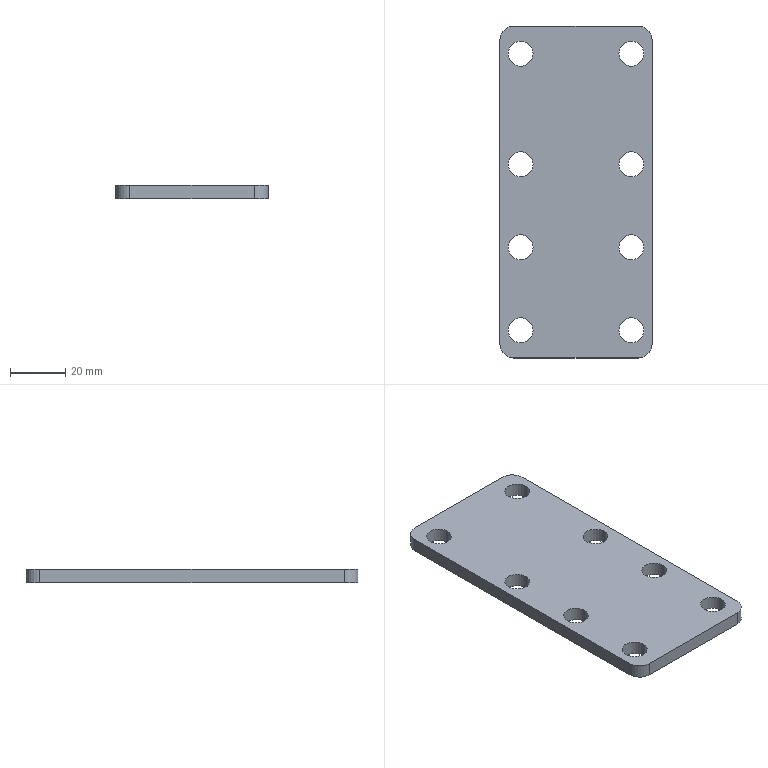Part | SolidWorks | features BaseBody 1 | 1 solid | 26 faces | box 55 x 120 x 5 mm | volume 30348 mm3 | cylinder 20 | plane 6 | commonest cylinder face diameters 9 x16 10 x4
STEP:
#1=CARTESIAN_POINT('',(3.,-10.,0.));
#2=VERTEX_POINT('',#1);
#3=CARTESIAN_POINT('',(12.,-10.,0.));
#4=VERTEX_POINT('',#3);
#5=CARTESIAN_POINT('',(7.5,-10.,0.));
#6=DIRECTION('',(0.,0.,1.));
#7=DIRECTION('',(1.,0.,0.));
#8=AXIS2_PLACEMENT_3D('',#5,#6,#7);
#9=CIRCLE('',#8,4.5);
#10=EDGE_CURVE('',#2,#4,#9,.T.);
#11=ORIENTED_EDGE('',*,*,#10,.F.);
#12=CARTESIAN_POINT('',(3.,-10.,5.));
#13=VERTEX_POINT('',#12);
#14=CARTESIAN_POINT('',(3.,-10.,5.));
#15=DIRECTION('',(0.,0.,1.));
#16=VECTOR('',#15,1000.);
#17=LINE('',#14,#16);
#18=EDGE_CURVE('',#2,#13,#17,.T.);
#19=ORIENTED_EDGE('',*,*,#18,.T.);
#20=CARTESIAN_POINT('',(12.,-10.,5.));
#21=VERTEX_POINT('',#20);
#22=CARTESIAN_POINT('',(7.5,-10.,5.));
#23=DIRECTION('',(0.,0.,1.));
#24=DIRECTION('',(1.,0.,0.));
#25=AXIS2_PLACEMENT_3D('',#22,#23,#24);
#26=CIRCLE('',#25,4.5);
#27=EDGE_CURVE('',#13,#21,#26,.T.);
#28=ORIENTED_EDGE('',*,*,#27,.T.);
#29=CARTESIAN_POINT('',(12.,-10.,5.));
#30=DIRECTION('',(0.,0.,1.));
#31=VECTOR('',#30,1000.);
#32=LINE('',#29,#31);
#33=EDGE_CURVE('',#4,#21,#32,.T.);
#34=ORIENTED_EDGE('',*,*,#33,.F.);
#35=EDGE_LOOP('',(#11,#19,#28,#34));
#36=FACE_OUTER_BOUND('',#35,.T.);
#37=CARTESIAN_POINT('',(7.5,-10.,5.));
#38=DIRECTION('',(0.,0.,1.));
#39=DIRECTION('',(1.,0.,0.));
#40=AXIS2_PLACEMENT_3D('',#37,#38,#39);
#41=CYLINDRICAL_SURFACE('',#40,4.5);
#42=ADVANCED_FACE('',(#36),#41,.F.);
#43=CARTESIAN_POINT('',(43.,-10.,0.));
#44=VERTEX_POINT('',#43);
#45=CARTESIAN_POINT('',(52.,-10.,0.));
#46=VERTEX_POINT('',#45);
#47=CARTESIAN_POINT('',(47.5,-10.,0.));
#48=DIRECTION('',(0.,0.,1.));
#49=DIRECTION('',(1.,0.,0.));
#50=AXIS2_PLACEMENT_3D('',#47,#48,#49);
#51=CIRCLE('',#50,4.5);
#52=EDGE_CURVE('',#44,#46,#51,.T.);
#53=ORIENTED_EDGE('',*,*,#52,.F.);
#54=CARTESIAN_POINT('',(43.,-10.,5.));
#55=VERTEX_POINT('',#54);
#56=CARTESIAN_POINT('',(43.,-10.,5.));
#57=DIRECTION('',(0.,0.,1.));
#58=VECTOR('',#57,1000.);
#59=LINE('',#56,#58);
#60=EDGE_CURVE('',#44,#55,#59,.T.);
#61=ORIENTED_EDGE('',*,*,#60,.T.);
#62=CARTESIAN_POINT('',(52.,-10.,5.));
#63=VERTEX_POINT('',#62);
#64=CARTESIAN_POINT('',(47.5,-10.,5.));
#65=DIRECTION('',(0.,0.,1.));
#66=DIRECTION('',(1.,0.,0.));
#67=AXIS2_PLACEMENT_3D('',#64,#65,#66);
#68=CIRCLE('',#67,4.5);
#69=EDGE_CURVE('',#55,#63,#68,.T.);
#70=ORIENTED_EDGE('',*,*,#69,.T.);
#71=CARTESIAN_POINT('',(52.,-10.,5.));
#72=DIRECTION('',(0.,0.,1.));
#73=VECTOR('',#72,1000.);
#74=LINE('',#71,#73);
#75=EDGE_CURVE('',#46,#63,#74,.T.);
#76=ORIENTED_EDGE('',*,*,#75,.F.);
#77=EDGE_LOOP('',(#53,#61,#70,#76));
#78=FACE_OUTER_BOUND('',#77,.T.);
#79=CARTESIAN_POINT('',(47.5,-10.,5.));
#80=DIRECTION('',(0.,0.,1.));
#81=DIRECTION('',(1.,0.,0.));
#82=AXIS2_PLACEMENT_3D('',#79,#80,#81);
#83=CYLINDRICAL_SURFACE('',#82,4.5);
#84=ADVANCED_FACE('',(#78),#83,.F.);
#85=CARTESIAN_POINT('',(3.,-50.,0.));
#86=VERTEX_POINT('',#85);
#87=CARTESIAN_POINT('',(12.,-50.,0.));
#88=VERTEX_POINT('',#87);
#89=CARTESIAN_POINT('',(7.5,-50.,0.));
#90=DIRECTION('',(0.,0.,1.));
#91=DIRECTION('',(1.,0.,0.));
#92=AXIS2_PLACEMENT_3D('',#89,#90,#91);
#93=CIRCLE('',#92,4.5);
#94=EDGE_CURVE('',#86,#88,#93,.T.);
#95=ORIENTED_EDGE('',*,*,#94,.F.);
#96=CARTESIAN_POINT('',(3.,-50.,5.));
#97=VERTEX_POINT('',#96);
#98=CARTESIAN_POINT('',(3.,-50.,5.));
#99=DIRECTION('',(0.,0.,1.));
#100=VECTOR('',#99,1000.);
#101=LINE('',#98,#100);
#102=EDGE_CURVE('',#86,#97,#101,.T.);
#103=ORIENTED_EDGE('',*,*,#102,.T.);
#104=CARTESIAN_POINT('',(12.,-50.,5.));
#105=VERTEX_POINT('',#104);
#106=CARTESIAN_POINT('',(7.5,-50.,5.));
#107=DIRECTION('',(0.,0.,1.));
#108=DIRECTION('',(1.,0.,0.));
#109=AXIS2_PLACEMENT_3D('',#106,#107,#108);
#110=CIRCLE('',#109,4.5);
#111=EDGE_CURVE('',#97,#105,#110,.T.);
#112=ORIENTED_EDGE('',*,*,#111,.T.);
#113=CARTESIAN_POINT('',(12.,-50.,5.));
#114=DIRECTION('',(0.,0.,1.));
#115=VECTOR('',#114,1000.);
#116=LINE('',#113,#115);
#117=EDGE_CURVE('',#88,#105,#116,.T.);
#118=ORIENTED_EDGE('',*,*,#117,.F.);
#119=EDGE_LOOP('',(#95,#103,#112,#118));
#120=FACE_OUTER_BOUND('',#119,.T.);
#121=CARTESIAN_POINT('',(7.5,-50.,5.));
#122=DIRECTION('',(0.,0.,1.));
#123=DIRECTION('',(1.,0.,0.));
#124=AXIS2_PLACEMENT_3D('',#121,#122,#123);
#125=CYLINDRICAL_SURFACE('',#124,4.5);
#126=ADVANCED_FACE('',(#120),#125,.F.);
#127=CARTESIAN_POINT('',(43.,-50.,0.));
#128=VERTEX_POINT('',#127);
#129=CARTESIAN_POINT('',(52.,-50.,0.));
#130=VERTEX_POINT('',#129);
#131=CARTESIAN_POINT('',(47.5,-50.,0.));
#132=DIRECTION('',(0.,0.,1.));
#133=DIRECTION('',(1.,0.,0.));
#134=AXIS2_PLACEMENT_3D('',#131,#132,#133);
#135=CIRCLE('',#134,4.5);
#136=EDGE_CURVE('',#128,#130,#135,.T.);
#137=ORIENTED_EDGE('',*,*,#136,.F.);
#138=CARTESIAN_POINT('',(43.,-50.,5.));
#139=VERTEX_POINT('',#138);
#140=CARTESIAN_POINT('',(43.,-50.,5.));
#141=DIRECTION('',(0.,0.,1.));
#142=VECTOR('',#141,1000.);
#143=LINE('',#140,#142);
#144=EDGE_CURVE('',#128,#139,#143,.T.);
#145=ORIENTED_EDGE('',*,*,#144,.T.);
#146=CARTESIAN_POINT('',(52.,-50.,5.));
#147=VERTEX_POINT('',#146);
#148=CARTESIAN_POINT('',(47.5,-50.,5.));
#149=DIRECTION('',(0.,0.,1.));
#150=DIRECTION('',(1.,0.,0.));
#151=AXIS2_PLACEMENT_3D('',#148,#149,#150);
#152=CIRCLE('',#151,4.5);
#153=EDGE_CURVE('',#139,#147,#152,.T.);
#154=ORIENTED_EDGE('',*,*,#153,.T.);
#155=CARTESIAN_POINT('',(52.,-50.,5.));
#156=DIRECTION('',(0.,0.,1.));
#157=VECTOR('',#156,1000.);
#158=LINE('',#155,#157);
#159=EDGE_CURVE('',#130,#147,#158,.T.);
#160=ORIENTED_EDGE('',*,*,#159,.F.);
#161=EDGE_LOOP('',(#137,#145,#154,#160));
#162=FACE_OUTER_BOUND('',#161,.T.);
#163=CARTESIAN_POINT('',(47.5,-50.,5.));
#164=DIRECTION('',(0.,0.,1.));
#165=DIRECTION('',(1.,0.,0.));
#166=AXIS2_PLACEMENT_3D('',#163,#164,#165);
#167=CYLINDRICAL_SURFACE('',#166,4.5);
#168=ADVANCED_FACE('',(#162),#167,.F.);
#169=CARTESIAN_POINT('',(43.,-110.,0.));
#170=VERTEX_POINT('',#169);
#171=CARTESIAN_POINT('',(52.,-110.,0.));
#172=VERTEX_POINT('',#171);
#173=CARTESIAN_POINT('',(47.5,-110.,0.));
#174=DIRECTION('',(0.,0.,1.));
#175=DIRECTION('',(1.,0.,0.));
#176=AXIS2_PLACEMENT_3D('',#173,#174,#175);
#177=CIRCLE('',#176,4.5);
#178=EDGE_CURVE('',#170,#172,#177,.T.);
#179=ORIENTED_EDGE('',*,*,#178,.F.);
#180=CARTESIAN_POINT('',(43.,-110.,5.));
#181=VERTEX_POINT('',#180);
#182=CARTESIAN_POINT('',(43.,-110.,5.));
#183=DIRECTION('',(0.,0.,1.));
#184=VECTOR('',#183,1000.);
#185=LINE('',#182,#184);
#186=EDGE_CURVE('',#170,#181,#185,.T.);
#187=ORIENTED_EDGE('',*,*,#186,.T.);
#188=CARTESIAN_POINT('',(52.,-110.,5.));
#189=VERTEX_POINT('',#188);
#190=CARTESIAN_POINT('',(47.5,-110.,5.));
#191=DIRECTION('',(0.,0.,1.));
#192=DIRECTION('',(1.,0.,0.));
#193=AXIS2_PLACEMENT_3D('',#190,#191,#192);
#194=CIRCLE('',#193,4.5);
#195=EDGE_CURVE('',#181,#189,#194,.T.);
#196=ORIENTED_EDGE('',*,*,#195,.T.);
#197=CARTESIAN_POINT('',(52.,-110.,5.));
#198=DIRECTION('',(0.,0.,1.));
#199=VECTOR('',#198,1000.);
#200=LINE('',#197,#199);
#201=EDGE_CURVE('',#172,#189,#200,.T.);
#202=ORIENTED_EDGE('',*,*,#201,.F.);
#203=EDGE_LOOP('',(#179,#187,#196,#202));
#204=FACE_OUTER_BOUND('',#203,.T.);
#205=CARTESIAN_POINT('',(47.5,-110.,5.));
#206=DIRECTION('',(0.,0.,1.));
#207=DIRECTION('',(1.,0.,0.));
#208=AXIS2_PLACEMENT_3D('',#205,#206,#207);
#209=CYLINDRICAL_SURFACE('',#208,4.5);
#210=ADVANCED_FACE('',(#204),#209,.F.);
#211=CARTESIAN_POINT('',(3.,-110.,0.));
#212=VERTEX_POINT('',#211);
#213=CARTESIAN_POINT('',(12.,-110.,0.));
#214=VERTEX_POINT('',#213);
#215=CARTESIAN_POINT('',(7.5,-110.,0.));
#216=DIRECTION('',(0.,0.,1.));
#217=DIRECTION('',(1.,0.,0.));
#218=AXIS2_PLACEMENT_3D('',#215,#216,#217);
#219=CIRCLE('',#218,4.5);
#220=EDGE_CURVE('',#212,#214,#219,.T.);
#221=ORIENTED_EDGE('',*,*,#220,.F.);
#222=CARTESIAN_POINT('',(3.,-110.,5.));
#223=VERTEX_POINT('',#222);
#224=CARTESIAN_POINT('',(3.,-110.,5.));
#225=DIRECTION('',(0.,0.,1.));
#226=VECTOR('',#225,1000.);
#227=LINE('',#224,#226);
#228=EDGE_CURVE('',#212,#223,#227,.T.);
#229=ORIENTED_EDGE('',*,*,#228,.T.);
#230=CARTESIAN_POINT('',(12.,-110.,5.));
#231=VERTEX_POINT('',#230);
#232=CARTESIAN_POINT('',(7.5,-110.,5.));
#233=DIRECTION('',(0.,0.,1.));
#234=DIRECTION('',(1.,0.,0.));
#235=AXIS2_PLACEMENT_3D('',#232,#233,#234);
#236=CIRCLE('',#235,4.5);
#237=EDGE_CURVE('',#223,#231,#236,.T.);
#238=ORIENTED_EDGE('',*,*,#237,.T.);
#239=CARTESIAN_POINT('',(12.,-110.,5.));
#240=DIRECTION('',(0.,0.,1.));
#241=VECTOR('',#240,1000.);
#242=LINE('',#239,#241);
#243=EDGE_CURVE('',#214,#231,#242,.T.);
#244=ORIENTED_EDGE('',*,*,#243,.F.);
#245=EDGE_LOOP('',(#221,#229,#238,#244));
#246=FACE_OUTER_BOUND('',#245,.T.);
#247=CARTESIAN_POINT('',(7.5,-110.,5.));
#248=DIRECTION('',(0.,0.,1.));
#249=DIRECTION('',(1.,0.,0.));
#250=AXIS2_PLACEMENT_3D('',#247,#248,#249);
#251=CYLINDRICAL_SURFACE('',#250,4.5);
#252=ADVANCED_FACE('',(#246),#251,.F.);
#253=CARTESIAN_POINT('',(43.,-80.,0.));
#254=VERTEX_POINT('',#253);
#255=CARTESIAN_POINT('',(52.,-80.,0.));
#256=VERTEX_POINT('',#255);
#257=CARTESIAN_POINT('',(47.5,-80.,0.));
#258=DIRECTION('',(0.,0.,1.));
#259=DIRECTION('',(1.,0.,0.));
#260=AXIS2_PLACEMENT_3D('',#257,#258,#259);
#261=CIRCLE('',#260,4.5);
#262=EDGE_CURVE('',#254,#256,#261,.T.);
#263=ORIENTED_EDGE('',*,*,#262,.F.);
#264=CARTESIAN_POINT('',(43.,-80.,5.));
#265=VERTEX_POINT('',#264);
#266=CARTESIAN_POINT('',(43.,-80.,5.));
#267=DIRECTION('',(0.,0.,1.));
#268=VECTOR('',#267,1000.);
#269=LINE('',#266,#268);
#270=EDGE_CURVE('',#254,#265,#269,.T.);
#271=ORIENTED_EDGE('',*,*,#270,.T.);
#272=CARTESIAN_POINT('',(52.,-80.,5.));
#273=VERTEX_POINT('',#272);
#274=CARTESIAN_POINT('',(47.5,-80.,5.));
#275=DIRECTION('',(0.,0.,1.));
#276=DIRECTION('',(1.,0.,0.));
#277=AXIS2_PLACEMENT_3D('',#274,#275,#276);
#278=CIRCLE('',#277,4.5);
#279=EDGE_CURVE('',#265,#273,#278,.T.);
#280=ORIENTED_EDGE('',*,*,#279,.T.);
#281=CARTESIAN_POINT('',(52.,-80.,5.));
#282=DIRECTION('',(0.,0.,1.));
#283=VECTOR('',#282,1000.);
#284=LINE('',#281,#283);
#285=EDGE_CURVE('',#256,#273,#284,.T.);
#286=ORIENTED_EDGE('',*,*,#285,.F.);
#287=EDGE_LOOP('',(#263,#271,#280,#286));
#288=FACE_OUTER_BOUND('',#287,.T.);
#289=CARTESIAN_POINT('',(47.5,-80.,5.));
#290=DIRECTION('',(0.,0.,1.));
#291=DIRECTION('',(1.,0.,0.));
#292=AXIS2_PLACEMENT_3D('',#289,#290,#291);
#293=CYLINDRICAL_SURFACE('',#292,4.5);
#294=ADVANCED_FACE('',(#288),#293,.F.);
#295=CARTESIAN_POINT('',(3.,-80.,0.));
#296=VERTEX_POINT('',#295);
#297=CARTESIAN_POINT('',(12.,-80.,0.));
#298=VERTEX_POINT('',#297);
#299=CARTESIAN_POINT('',(7.5,-80.,0.));
#300=DIRECTION('',(0.,0.,1.));
#301=DIRECTION('',(1.,0.,0.));
#302=AXIS2_PLACEMENT_3D('',#299,#300,#301);
#303=CIRCLE('',#302,4.5);
#304=EDGE_CURVE('',#296,#298,#303,.T.);
#305=ORIENTED_EDGE('',*,*,#304,.F.);
#306=CARTESIAN_POINT('',(3.,-80.,5.));
#307=VERTEX_POINT('',#306);
#308=CARTESIAN_POINT('',(3.,-80.,5.));
#309=DIRECTION('',(0.,0.,1.));
#310=VECTOR('',#309,1000.);
#311=LINE('',#308,#310);
#312=EDGE_CURVE('',#296,#307,#311,.T.);
#313=ORIENTED_EDGE('',*,*,#312,.T.);
#314=CARTESIAN_POINT('',(12.,-80.,5.));
#315=VERTEX_POINT('',#314);
#316=CARTESIAN_POINT('',(7.5,-80.,5.));
#317=DIRECTION('',(0.,0.,1.));
#318=DIRECTION('',(1.,0.,0.));
#319=AXIS2_PLACEMENT_3D('',#316,#317,#318);
#320=CIRCLE('',#319,4.5);
#321=EDGE_CURVE('',#307,#315,#320,.T.);
#322=ORIENTED_EDGE('',*,*,#321,.T.);
#323=CARTESIAN_POINT('',(12.,-80.,5.));
#324=DIRECTION('',(0.,0.,1.));
#325=VECTOR('',#324,1000.);
#326=LINE('',#323,#325);
#327=EDGE_CURVE('',#298,#315,#326,.T.);
#328=ORIENTED_EDGE('',*,*,#327,.F.);
#329=EDGE_LOOP('',(#305,#313,#322,#328));
#330=FACE_OUTER_BOUND('',#329,.T.);
#331=CARTESIAN_POINT('',(7.5,-80.,5.));
#332=DIRECTION('',(0.,0.,1.));
#333=DIRECTION('',(1.,0.,0.));
#334=AXIS2_PLACEMENT_3D('',#331,#332,#333);
#335=CYLINDRICAL_SURFACE('',#334,4.5);
#336=ADVANCED_FACE('',(#330),#335,.F.);
#337=CARTESIAN_POINT('',(0.,-5.,0.));
#338=VERTEX_POINT('',#337);
#339=CARTESIAN_POINT('',(0.,-115.,0.));
#340=VERTEX_POINT('',#339);
#341=CARTESIAN_POINT('',(0.,0.,0.));
#342=DIRECTION('',(0.,-1.,0.));
#343=VECTOR('',#342,1000.);
#344=LINE('',#341,#343);
#345=EDGE_CURVE('',#338,#340,#344,.T.);
#346=ORIENTED_EDGE('',*,*,#345,.T.);
#347=CARTESIAN_POINT('',(0.,-115.,5.));
#348=VERTEX_POINT('',#347);
#349=CARTESIAN_POINT('',(0.,-115.,5.));
#350=DIRECTION('',(0.,0.,1.));
#351=VECTOR('',#350,1000.);
#352=LINE('',#349,#351);
#353=EDGE_CURVE('',#340,#348,#352,.T.);
#354=ORIENTED_EDGE('',*,*,#353,.T.);
#355=CARTESIAN_POINT('',(0.,-5.,5.));
#356=VERTEX_POINT('',#355);
#357=CARTESIAN_POINT('',(0.,0.,5.));
#358=DIRECTION('',(0.,-1.,0.));
#359=VECTOR('',#358,1000.);
#360=LINE('',#357,#359);
#361=EDGE_CURVE('',#356,#348,#360,.T.);
#362=ORIENTED_EDGE('',*,*,#361,.F.);
#363=CARTESIAN_POINT('',(0.,-5.,5.));
#364=DIRECTION('',(0.,0.,-1.));
#365=VECTOR('',#364,1000.);
#366=LINE('',#363,#365);
#367=EDGE_CURVE('',#356,#338,#366,.T.);
#368=ORIENTED_EDGE('',*,*,#367,.T.);
#369=EDGE_LOOP('',(#346,#354,#362,#368));
#370=FACE_OUTER_BOUND('',#369,.T.);
#371=CARTESIAN_POINT('',(0.,0.,5.));
#372=DIRECTION('',(1.,0.,0.));
#373=DIRECTION('',(0.,1.,0.));
#374=AXIS2_PLACEMENT_3D('',#371,#372,#373);
#375=PLANE('',#374);
#376=ADVANCED_FACE('',(#370),#375,.F.);
#377=CARTESIAN_POINT('',(5.,-120.,5.));
#378=VERTEX_POINT('',#377);
#379=CARTESIAN_POINT('',(50.,-120.,5.));
#380=VERTEX_POINT('',#379);
#381=CARTESIAN_POINT('',(0.,-120.,5.));
#382=DIRECTION('',(1.,0.,0.));
#383=VECTOR('',#382,1000.);
#384=LINE('',#381,#383);
#385=EDGE_CURVE('',#378,#380,#384,.T.);
#386=ORIENTED_EDGE('',*,*,#385,.F.);
#387=CARTESIAN_POINT('',(5.,-120.,0.));
#388=VERTEX_POINT('',#387);
#389=CARTESIAN_POINT('',(5.,-120.,5.));
#390=DIRECTION('',(0.,0.,-1.));
#391=VECTOR('',#390,1000.);
#392=LINE('',#389,#391);
#393=EDGE_CURVE('',#378,#388,#392,.T.);
#394=ORIENTED_EDGE('',*,*,#393,.T.);
#395=CARTESIAN_POINT('',(50.,-120.,0.));
#396=VERTEX_POINT('',#395);
#397=CARTESIAN_POINT('',(0.,-120.,0.));
#398=DIRECTION('',(1.,0.,0.));
#399=VECTOR('',#398,1000.);
#400=LINE('',#397,#399);
#401=EDGE_CURVE('',#388,#396,#400,.T.);
#402=ORIENTED_EDGE('',*,*,#401,.T.);
#403=CARTESIAN_POINT('',(50.,-120.,5.));
#404=DIRECTION('',(0.,0.,1.));
#405=VECTOR('',#404,1000.);
#406=LINE('',#403,#405);
#407=EDGE_CURVE('',#396,#380,#406,.T.);
#408=ORIENTED_EDGE('',*,*,#407,.T.);
#409=EDGE_LOOP('',(#386,#394,#402,#408));
#410=FACE_OUTER_BOUND('',#409,.T.);
#411=CARTESIAN_POINT('',(0.,-120.,5.));
#412=DIRECTION('',(0.,1.,0.));
#413=DIRECTION('',(0.,0.,1.));
#414=AXIS2_PLACEMENT_3D('',#411,#412,#413);
#415=PLANE('',#414);
#416=ADVANCED_FACE('',(#410),#415,.F.);
#417=CARTESIAN_POINT('',(55.,-115.,5.));
#418=VERTEX_POINT('',#417);
#419=CARTESIAN_POINT('',(55.,-5.,5.));
#420=VERTEX_POINT('',#419);
#421=CARTESIAN_POINT('',(55.,0.,5.));
#422=DIRECTION('',(0.,1.,0.));
#423=VECTOR('',#422,1000.);
#424=LINE('',#421,#423);
#425=EDGE_CURVE('',#418,#420,#424,.T.);
#426=ORIENTED_EDGE('',*,*,#425,.F.);
#427=CARTESIAN_POINT('',(55.,-115.,0.));
#428=VERTEX_POINT('',#427);
#429=CARTESIAN_POINT('',(55.,-115.,5.));
#430=DIRECTION('',(0.,0.,-1.));
#431=VECTOR('',#430,1000.);
#432=LINE('',#429,#431);
#433=EDGE_CURVE('',#418,#428,#432,.T.);
#434=ORIENTED_EDGE('',*,*,#433,.T.);
#435=CARTESIAN_POINT('',(55.,-5.,0.));
#436=VERTEX_POINT('',#435);
#437=CARTESIAN_POINT('',(55.,0.,0.));
#438=DIRECTION('',(0.,1.,0.));
#439=VECTOR('',#438,1000.);
#440=LINE('',#437,#439);
#441=EDGE_CURVE('',#428,#436,#440,.T.);
#442=ORIENTED_EDGE('',*,*,#441,.T.);
#443=CARTESIAN_POINT('',(55.,-5.,5.));
#444=DIRECTION('',(0.,0.,1.));
#445=VECTOR('',#444,1000.);
#446=LINE('',#443,#445);
#447=EDGE_CURVE('',#436,#420,#446,.T.);
#448=ORIENTED_EDGE('',*,*,#447,.T.);
#449=EDGE_LOOP('',(#426,#434,#442,#448));
#450=FACE_OUTER_BOUND('',#449,.T.);
#451=CARTESIAN_POINT('',(55.,0.,5.));
#452=DIRECTION('',(-1.,0.,0.));
#453=DIRECTION('',(0.,-1.,0.));
#454=AXIS2_PLACEMENT_3D('',#451,#452,#453);
#455=PLANE('',#454);
#456=ADVANCED_FACE('',(#450),#455,.F.);
#457=CARTESIAN_POINT('',(50.,0.,5.));
#458=VERTEX_POINT('',#457);
#459=CARTESIAN_POINT('',(5.,0.,5.));
#460=VERTEX_POINT('',#459);
#461=CARTESIAN_POINT('',(0.,0.,5.));
#462=DIRECTION('',(-1.,0.,0.));
#463=VECTOR('',#462,1000.);
#464=LINE('',#461,#463);
#465=EDGE_CURVE('',#458,#460,#464,.T.);
#466=ORIENTED_EDGE('',*,*,#465,.F.);
#467=CARTESIAN_POINT('',(50.,0.,0.));
#468=VERTEX_POINT('',#467);
#469=CARTESIAN_POINT('',(50.,0.,5.));
#470=DIRECTION('',(0.,0.,-1.));
#471=VECTOR('',#470,1000.);
#472=LINE('',#469,#471);
#473=EDGE_CURVE('',#458,#468,#472,.T.);
#474=ORIENTED_EDGE('',*,*,#473,.T.);
#475=CARTESIAN_POINT('',(5.,0.,0.));
#476=VERTEX_POINT('',#475);
#477=CARTESIAN_POINT('',(0.,0.,0.));
#478=DIRECTION('',(-1.,0.,0.));
#479=VECTOR('',#478,1000.);
#480=LINE('',#477,#479);
#481=EDGE_CURVE('',#468,#476,#480,.T.);
#482=ORIENTED_EDGE('',*,*,#481,.T.);
#483=CARTESIAN_POINT('',(5.,0.,5.));
#484=DIRECTION('',(0.,0.,1.));
#485=VECTOR('',#484,1000.);
#486=LINE('',#483,#485);
#487=EDGE_CURVE('',#476,#460,#486,.T.);
#488=ORIENTED_EDGE('',*,*,#487,.T.);
#489=EDGE_LOOP('',(#466,#474,#482,#488));
#490=FACE_OUTER_BOUND('',#489,.T.);
#491=CARTESIAN_POINT('',(0.,0.,5.));
#492=DIRECTION('',(0.,-1.,0.));
#493=DIRECTION('',(0.,0.,-1.));
#494=AXIS2_PLACEMENT_3D('',#491,#492,#493);
#495=PLANE('',#494);
#496=ADVANCED_FACE('',(#490),#495,.F.);
#497=CARTESIAN_POINT('',(7.5,-10.,5.));
#498=DIRECTION('',(0.,0.,1.));
#499=DIRECTION('',(1.,0.,0.));
#500=AXIS2_PLACEMENT_3D('',#497,#498,#499);
#501=CIRCLE('',#500,4.5);
#502=EDGE_CURVE('',#21,#13,#501,.T.);
#503=ORIENTED_EDGE('',*,*,#502,.F.);
#504=ORIENTED_EDGE('',*,*,#27,.F.);
#505=EDGE_LOOP('',(#503,#504));
#506=FACE_BOUND('',#505,.T.);
#507=CARTESIAN_POINT('',(47.5,-10.,5.));
#508=DIRECTION('',(0.,0.,1.));
#509=DIRECTION('',(1.,0.,0.));
#510=AXIS2_PLACEMENT_3D('',#507,#508,#509);
#511=CIRCLE('',#510,4.5);
#512=EDGE_CURVE('',#63,#55,#511,.T.);
#513=ORIENTED_EDGE('',*,*,#512,.F.);
#514=ORIENTED_EDGE('',*,*,#69,.F.);
#515=EDGE_LOOP('',(#513,#514));
#516=FACE_BOUND('',#515,.T.);
#517=CARTESIAN_POINT('',(7.5,-50.,5.));
#518=DIRECTION('',(0.,0.,1.));
#519=DIRECTION('',(1.,0.,0.));
#520=AXIS2_PLACEMENT_3D('',#517,#518,#519);
#521=CIRCLE('',#520,4.5);
#522=EDGE_CURVE('',#105,#97,#521,.T.);
#523=ORIENTED_EDGE('',*,*,#522,.F.);
#524=ORIENTED_EDGE('',*,*,#111,.F.);
#525=EDGE_LOOP('',(#523,#524));
#526=FACE_BOUND('',#525,.T.);
#527=CARTESIAN_POINT('',(47.5,-50.,5.));
#528=DIRECTION('',(0.,0.,1.));
#529=DIRECTION('',(1.,0.,0.));
#530=AXIS2_PLACEMENT_3D('',#527,#528,#529);
#531=CIRCLE('',#530,4.5);
#532=EDGE_CURVE('',#147,#139,#531,.T.);
#533=ORIENTED_EDGE('',*,*,#532,.F.);
#534=ORIENTED_EDGE('',*,*,#153,.F.);
#535=EDGE_LOOP('',(#533,#534));
#536=FACE_BOUND('',#535,.T.);
#537=CARTESIAN_POINT('',(47.5,-110.,5.));
#538=DIRECTION('',(0.,0.,1.));
#539=DIRECTION('',(1.,0.,0.));
#540=AXIS2_PLACEMENT_3D('',#537,#538,#539);
#541=CIRCLE('',#540,4.5);
#542=EDGE_CURVE('',#189,#181,#541,.T.);
#543=ORIENTED_EDGE('',*,*,#542,.F.);
#544=ORIENTED_EDGE('',*,*,#195,.F.);
#545=EDGE_LOOP('',(#543,#544));
#546=FACE_BOUND('',#545,.T.);
#547=CARTESIAN_POINT('',(7.5,-110.,5.));
#548=DIRECTION('',(0.,0.,1.));
#549=DIRECTION('',(1.,0.,0.));
#550=AXIS2_PLACEMENT_3D('',#547,#548,#549);
#551=CIRCLE('',#550,4.5);
#552=EDGE_CURVE('',#231,#223,#551,.T.);
#553=ORIENTED_EDGE('',*,*,#552,.F.);
#554=ORIENTED_EDGE('',*,*,#237,.F.);
#555=EDGE_LOOP('',(#553,#554));
#556=FACE_BOUND('',#555,.T.);
#557=CARTESIAN_POINT('',(47.5,-80.,5.));
#558=DIRECTION('',(0.,0.,1.));
#559=DIRECTION('',(1.,0.,0.));
#560=AXIS2_PLACEMENT_3D('',#557,#558,#559);
#561=CIRCLE('',#560,4.5);
#562=EDGE_CURVE('',#273,#265,#561,.T.);
#563=ORIENTED_EDGE('',*,*,#562,.F.);
#564=ORIENTED_EDGE('',*,*,#279,.F.);
#565=EDGE_LOOP('',(#563,#564));
#566=FACE_BOUND('',#565,.T.);
#567=CARTESIAN_POINT('',(7.5,-80.,5.));
#568=DIRECTION('',(0.,0.,1.));
#569=DIRECTION('',(1.,0.,0.));
#570=AXIS2_PLACEMENT_3D('',#567,#568,#569);
#571=CIRCLE('',#570,4.5);
#572=EDGE_CURVE('',#315,#307,#571,.T.);
#573=ORIENTED_EDGE('',*,*,#572,.F.);
#574=ORIENTED_EDGE('',*,*,#321,.F.);
#575=EDGE_LOOP('',(#573,#574));
#576=FACE_BOUND('',#575,.T.);
#577=ORIENTED_EDGE('',*,*,#361,.T.);
#578=CARTESIAN_POINT('',(5.,-115.,5.));
#579=DIRECTION('',(0.,0.,1.));
#580=DIRECTION('',(1.,0.,0.));
#581=AXIS2_PLACEMENT_3D('',#578,#579,#580);
#582=CIRCLE('',#581,5.);
#583=EDGE_CURVE('',#348,#378,#582,.T.);
#584=ORIENTED_EDGE('',*,*,#583,.T.);
#585=ORIENTED_EDGE('',*,*,#385,.T.);
#586=CARTESIAN_POINT('',(50.,-115.,5.));
#587=DIRECTION('',(0.,0.,1.));
#588=DIRECTION('',(1.,0.,0.));
#589=AXIS2_PLACEMENT_3D('',#586,#587,#588);
#590=CIRCLE('',#589,5.);
#591=EDGE_CURVE('',#380,#418,#590,.T.);
#592=ORIENTED_EDGE('',*,*,#591,.T.);
#593=ORIENTED_EDGE('',*,*,#425,.T.);
#594=CARTESIAN_POINT('',(50.,-5.,5.));
#595=DIRECTION('',(0.,0.,1.));
#596=DIRECTION('',(1.,0.,0.));
#597=AXIS2_PLACEMENT_3D('',#594,#595,#596);
#598=CIRCLE('',#597,5.);
#599=EDGE_CURVE('',#420,#458,#598,.T.);
#600=ORIENTED_EDGE('',*,*,#599,.T.);
#601=ORIENTED_EDGE('',*,*,#465,.T.);
#602=CARTESIAN_POINT('',(5.,-5.,5.));
#603=DIRECTION('',(0.,0.,1.));
#604=DIRECTION('',(1.,0.,0.));
#605=AXIS2_PLACEMENT_3D('',#602,#603,#604);
#606=CIRCLE('',#605,5.);
#607=EDGE_CURVE('',#460,#356,#606,.T.);
#608=ORIENTED_EDGE('',*,*,#607,.T.);
#609=EDGE_LOOP('',(#577,#584,#585,#592,#593,#600,#601,#608));
#610=FACE_OUTER_BOUND('',#609,.T.);
#611=CARTESIAN_POINT('',(0.,0.,5.));
#612=DIRECTION('',(0.,0.,1.));
#613=DIRECTION('',(1.,0.,0.));
#614=AXIS2_PLACEMENT_3D('',#611,#612,#613);
#615=PLANE('',#614);
#616=ADVANCED_FACE('',(#506,#516,#526,#536,#546,#556,#566,#576,#610),#615,.T.);
#617=CARTESIAN_POINT('',(7.5,-10.,0.));
#618=DIRECTION('',(0.,0.,1.));
#619=DIRECTION('',(1.,0.,0.));
#620=AXIS2_PLACEMENT_3D('',#617,#618,#619);
#621=CIRCLE('',#620,4.5);
#622=EDGE_CURVE('',#4,#2,#621,.T.);
#623=ORIENTED_EDGE('',*,*,#622,.T.);
#624=ORIENTED_EDGE('',*,*,#10,.T.);
#625=EDGE_LOOP('',(#623,#624));
#626=FACE_BOUND('',#625,.T.);
#627=CARTESIAN_POINT('',(47.5,-10.,0.));
#628=DIRECTION('',(0.,0.,1.));
#629=DIRECTION('',(1.,0.,0.));
#630=AXIS2_PLACEMENT_3D('',#627,#628,#629);
#631=CIRCLE('',#630,4.5);
#632=EDGE_CURVE('',#46,#44,#631,.T.);
#633=ORIENTED_EDGE('',*,*,#632,.T.);
#634=ORIENTED_EDGE('',*,*,#52,.T.);
#635=EDGE_LOOP('',(#633,#634));
#636=FACE_BOUND('',#635,.T.);
#637=CARTESIAN_POINT('',(7.5,-50.,0.));
#638=DIRECTION('',(0.,0.,1.));
#639=DIRECTION('',(1.,0.,0.));
#640=AXIS2_PLACEMENT_3D('',#637,#638,#639);
#641=CIRCLE('',#640,4.5);
#642=EDGE_CURVE('',#88,#86,#641,.T.);
#643=ORIENTED_EDGE('',*,*,#642,.T.);
#644=ORIENTED_EDGE('',*,*,#94,.T.);
#645=EDGE_LOOP('',(#643,#644));
#646=FACE_BOUND('',#645,.T.);
#647=CARTESIAN_POINT('',(47.5,-50.,0.));
#648=DIRECTION('',(0.,0.,1.));
#649=DIRECTION('',(1.,0.,0.));
#650=AXIS2_PLACEMENT_3D('',#647,#648,#649);
#651=CIRCLE('',#650,4.5);
#652=EDGE_CURVE('',#130,#128,#651,.T.);
#653=ORIENTED_EDGE('',*,*,#652,.T.);
#654=ORIENTED_EDGE('',*,*,#136,.T.);
#655=EDGE_LOOP('',(#653,#654));
#656=FACE_BOUND('',#655,.T.);
#657=CARTESIAN_POINT('',(47.5,-110.,0.));
#658=DIRECTION('',(0.,0.,1.));
#659=DIRECTION('',(1.,0.,0.));
#660=AXIS2_PLACEMENT_3D('',#657,#658,#659);
#661=CIRCLE('',#660,4.5);
#662=EDGE_CURVE('',#172,#170,#661,.T.);
#663=ORIENTED_EDGE('',*,*,#662,.T.);
#664=ORIENTED_EDGE('',*,*,#178,.T.);
#665=EDGE_LOOP('',(#663,#664));
#666=FACE_BOUND('',#665,.T.);
#667=CARTESIAN_POINT('',(7.5,-110.,0.));
#668=DIRECTION('',(0.,0.,1.));
#669=DIRECTION('',(1.,0.,0.));
#670=AXIS2_PLACEMENT_3D('',#667,#668,#669);
#671=CIRCLE('',#670,4.5);
#672=EDGE_CURVE('',#214,#212,#671,.T.);
#673=ORIENTED_EDGE('',*,*,#672,.T.);
#674=ORIENTED_EDGE('',*,*,#220,.T.);
#675=EDGE_LOOP('',(#673,#674));
#676=FACE_BOUND('',#675,.T.);
#677=CARTESIAN_POINT('',(47.5,-80.,0.));
#678=DIRECTION('',(0.,0.,1.));
#679=DIRECTION('',(1.,0.,0.));
#680=AXIS2_PLACEMENT_3D('',#677,#678,#679);
#681=CIRCLE('',#680,4.5);
#682=EDGE_CURVE('',#256,#254,#681,.T.);
#683=ORIENTED_EDGE('',*,*,#682,.T.);
#684=ORIENTED_EDGE('',*,*,#262,.T.);
#685=EDGE_LOOP('',(#683,#684));
#686=FACE_BOUND('',#685,.T.);
#687=CARTESIAN_POINT('',(7.5,-80.,0.));
#688=DIRECTION('',(0.,0.,1.));
#689=DIRECTION('',(1.,0.,0.));
#690=AXIS2_PLACEMENT_3D('',#687,#688,#689);
#691=CIRCLE('',#690,4.5);
#692=EDGE_CURVE('',#298,#296,#691,.T.);
#693=ORIENTED_EDGE('',*,*,#692,.T.);
#694=ORIENTED_EDGE('',*,*,#304,.T.);
#695=EDGE_LOOP('',(#693,#694));
#696=FACE_BOUND('',#695,.T.);
#697=ORIENTED_EDGE('',*,*,#401,.F.);
#698=CARTESIAN_POINT('',(5.,-115.,0.));
#699=DIRECTION('',(0.,0.,-1.));
#700=DIRECTION('',(1.,0.,0.));
#701=AXIS2_PLACEMENT_3D('',#698,#699,#700);
#702=CIRCLE('',#701,5.);
#703=EDGE_CURVE('',#388,#340,#702,.T.);
#704=ORIENTED_EDGE('',*,*,#703,.T.);
#705=ORIENTED_EDGE('',*,*,#345,.F.);
#706=CARTESIAN_POINT('',(5.,-5.,0.));
#707=DIRECTION('',(0.,0.,-1.));
#708=DIRECTION('',(1.,0.,0.));
#709=AXIS2_PLACEMENT_3D('',#706,#707,#708);
#710=CIRCLE('',#709,5.);
#711=EDGE_CURVE('',#338,#476,#710,.T.);
#712=ORIENTED_EDGE('',*,*,#711,.T.);
#713=ORIENTED_EDGE('',*,*,#481,.F.);
#714=CARTESIAN_POINT('',(50.,-5.,0.));
#715=DIRECTION('',(0.,0.,-1.));
#716=DIRECTION('',(1.,0.,0.));
#717=AXIS2_PLACEMENT_3D('',#714,#715,#716);
#718=CIRCLE('',#717,5.);
#719=EDGE_CURVE('',#468,#436,#718,.T.);
#720=ORIENTED_EDGE('',*,*,#719,.T.);
#721=ORIENTED_EDGE('',*,*,#441,.F.);
#722=CARTESIAN_POINT('',(50.,-115.,0.));
#723=DIRECTION('',(0.,0.,-1.));
#724=DIRECTION('',(1.,0.,0.));
#725=AXIS2_PLACEMENT_3D('',#722,#723,#724);
#726=CIRCLE('',#725,5.);
#727=EDGE_CURVE('',#428,#396,#726,.T.);
#728=ORIENTED_EDGE('',*,*,#727,.T.);
#729=EDGE_LOOP('',(#697,#704,#705,#712,#713,#720,#721,#728));
#730=FACE_OUTER_BOUND('',#729,.T.);
#731=CARTESIAN_POINT('',(0.,0.,0.));
#732=DIRECTION('',(0.,0.,1.));
#733=DIRECTION('',(1.,0.,0.));
#734=AXIS2_PLACEMENT_3D('',#731,#732,#733);
#735=PLANE('',#734);
#736=ADVANCED_FACE('',(#626,#636,#646,#656,#666,#676,#686,#696,#730),#735,.F.);
#737=ORIENTED_EDGE('',*,*,#312,.F.);
#738=ORIENTED_EDGE('',*,*,#692,.F.);
#739=ORIENTED_EDGE('',*,*,#327,.T.);
#740=ORIENTED_EDGE('',*,*,#572,.T.);
#741=EDGE_LOOP('',(#737,#738,#739,#740));
#742=FACE_OUTER_BOUND('',#741,.T.);
#743=CARTESIAN_POINT('',(7.5,-80.,5.));
#744=DIRECTION('',(0.,0.,1.));
#745=DIRECTION('',(1.,0.,0.));
#746=AXIS2_PLACEMENT_3D('',#743,#744,#745);
#747=CYLINDRICAL_SURFACE('',#746,4.5);
#748=ADVANCED_FACE('',(#742),#747,.F.);
#749=ORIENTED_EDGE('',*,*,#270,.F.);
#750=ORIENTED_EDGE('',*,*,#682,.F.);
#751=ORIENTED_EDGE('',*,*,#285,.T.);
#752=ORIENTED_EDGE('',*,*,#562,.T.);
#753=EDGE_LOOP('',(#749,#750,#751,#752));
#754=FACE_OUTER_BOUND('',#753,.T.);
#755=CARTESIAN_POINT('',(47.5,-80.,5.));
#756=DIRECTION('',(0.,0.,1.));
#757=DIRECTION('',(1.,0.,0.));
#758=AXIS2_PLACEMENT_3D('',#755,#756,#757);
#759=CYLINDRICAL_SURFACE('',#758,4.5);
#760=ADVANCED_FACE('',(#754),#759,.F.);
#761=ORIENTED_EDGE('',*,*,#228,.F.);
#762=ORIENTED_EDGE('',*,*,#672,.F.);
#763=ORIENTED_EDGE('',*,*,#243,.T.);
#764=ORIENTED_EDGE('',*,*,#552,.T.);
#765=EDGE_LOOP('',(#761,#762,#763,#764));
#766=FACE_OUTER_BOUND('',#765,.T.);
#767=CARTESIAN_POINT('',(7.5,-110.,5.));
#768=DIRECTION('',(0.,0.,1.));
#769=DIRECTION('',(1.,0.,0.));
#770=AXIS2_PLACEMENT_3D('',#767,#768,#769);
#771=CYLINDRICAL_SURFACE('',#770,4.5);
#772=ADVANCED_FACE('',(#766),#771,.F.);
#773=ORIENTED_EDGE('',*,*,#186,.F.);
#774=ORIENTED_EDGE('',*,*,#662,.F.);
#775=ORIENTED_EDGE('',*,*,#201,.T.);
#776=ORIENTED_EDGE('',*,*,#542,.T.);
#777=EDGE_LOOP('',(#773,#774,#775,#776));
#778=FACE_OUTER_BOUND('',#777,.T.);
#779=CARTESIAN_POINT('',(47.5,-110.,5.));
#780=DIRECTION('',(0.,0.,1.));
#781=DIRECTION('',(1.,0.,0.));
#782=AXIS2_PLACEMENT_3D('',#779,#780,#781);
#783=CYLINDRICAL_SURFACE('',#782,4.5);
#784=ADVANCED_FACE('',(#778),#783,.F.);
#785=ORIENTED_EDGE('',*,*,#144,.F.);
#786=ORIENTED_EDGE('',*,*,#652,.F.);
#787=ORIENTED_EDGE('',*,*,#159,.T.);
#788=ORIENTED_EDGE('',*,*,#532,.T.);
#789=EDGE_LOOP('',(#785,#786,#787,#788));
#790=FACE_OUTER_BOUND('',#789,.T.);
#791=CARTESIAN_POINT('',(47.5,-50.,5.));
#792=DIRECTION('',(0.,0.,1.));
#793=DIRECTION('',(1.,0.,0.));
#794=AXIS2_PLACEMENT_3D('',#791,#792,#793);
#795=CYLINDRICAL_SURFACE('',#794,4.5);
#796=ADVANCED_FACE('',(#790),#795,.F.);
#797=ORIENTED_EDGE('',*,*,#102,.F.);
#798=ORIENTED_EDGE('',*,*,#642,.F.);
#799=ORIENTED_EDGE('',*,*,#117,.T.);
#800=ORIENTED_EDGE('',*,*,#522,.T.);
#801=EDGE_LOOP('',(#797,#798,#799,#800));
#802=FACE_OUTER_BOUND('',#801,.T.);
#803=CARTESIAN_POINT('',(7.5,-50.,5.));
#804=DIRECTION('',(0.,0.,1.));
#805=DIRECTION('',(1.,0.,0.));
#806=AXIS2_PLACEMENT_3D('',#803,#804,#805);
#807=CYLINDRICAL_SURFACE('',#806,4.5);
#808=ADVANCED_FACE('',(#802),#807,.F.);
#809=ORIENTED_EDGE('',*,*,#60,.F.);
#810=ORIENTED_EDGE('',*,*,#632,.F.);
#811=ORIENTED_EDGE('',*,*,#75,.T.);
#812=ORIENTED_EDGE('',*,*,#512,.T.);
#813=EDGE_LOOP('',(#809,#810,#811,#812));
#814=FACE_OUTER_BOUND('',#813,.T.);
#815=CARTESIAN_POINT('',(47.5,-10.,5.));
#816=DIRECTION('',(0.,0.,1.));
#817=DIRECTION('',(1.,0.,0.));
#818=AXIS2_PLACEMENT_3D('',#815,#816,#817);
#819=CYLINDRICAL_SURFACE('',#818,4.5);
#820=ADVANCED_FACE('',(#814),#819,.F.);
#821=ORIENTED_EDGE('',*,*,#18,.F.);
#822=ORIENTED_EDGE('',*,*,#622,.F.);
#823=ORIENTED_EDGE('',*,*,#33,.T.);
#824=ORIENTED_EDGE('',*,*,#502,.T.);
#825=EDGE_LOOP('',(#821,#822,#823,#824));
#826=FACE_OUTER_BOUND('',#825,.T.);
#827=CARTESIAN_POINT('',(7.5,-10.,5.));
#828=DIRECTION('',(0.,0.,1.));
#829=DIRECTION('',(1.,0.,0.));
#830=AXIS2_PLACEMENT_3D('',#827,#828,#829);
#831=CYLINDRICAL_SURFACE('',#830,4.5);
#832=ADVANCED_FACE('',(#826),#831,.F.);
#833=ORIENTED_EDGE('',*,*,#583,.F.);
#834=ORIENTED_EDGE('',*,*,#353,.F.);
#835=ORIENTED_EDGE('',*,*,#703,.F.);
#836=ORIENTED_EDGE('',*,*,#393,.F.);
#837=EDGE_LOOP('',(#833,#834,#835,#836));
#838=FACE_OUTER_BOUND('',#837,.T.);
#839=CARTESIAN_POINT('',(5.,-115.,5.));
#840=DIRECTION('',(0.,0.,-1.));
#841=DIRECTION('',(-1.,0.,0.));
#842=AXIS2_PLACEMENT_3D('',#839,#840,#841);
#843=CYLINDRICAL_SURFACE('',#842,5.);
#844=ADVANCED_FACE('',(#838),#843,.T.);
#845=ORIENTED_EDGE('',*,*,#591,.F.);
#846=ORIENTED_EDGE('',*,*,#407,.F.);
#847=ORIENTED_EDGE('',*,*,#727,.F.);
#848=ORIENTED_EDGE('',*,*,#433,.F.);
#849=EDGE_LOOP('',(#845,#846,#847,#848));
#850=FACE_OUTER_BOUND('',#849,.T.);
#851=CARTESIAN_POINT('',(50.,-115.,5.));
#852=DIRECTION('',(0.,0.,-1.));
#853=DIRECTION('',(-1.,0.,0.));
#854=AXIS2_PLACEMENT_3D('',#851,#852,#853);
#855=CYLINDRICAL_SURFACE('',#854,5.);
#856=ADVANCED_FACE('',(#850),#855,.T.);
#857=ORIENTED_EDGE('',*,*,#599,.F.);
#858=ORIENTED_EDGE('',*,*,#447,.F.);
#859=ORIENTED_EDGE('',*,*,#719,.F.);
#860=ORIENTED_EDGE('',*,*,#473,.F.);
#861=EDGE_LOOP('',(#857,#858,#859,#860));
#862=FACE_OUTER_BOUND('',#861,.T.);
#863=CARTESIAN_POINT('',(50.,-5.,5.));
#864=DIRECTION('',(0.,0.,-1.));
#865=DIRECTION('',(-1.,0.,0.));
#866=AXIS2_PLACEMENT_3D('',#863,#864,#865);
#867=CYLINDRICAL_SURFACE('',#866,5.);
#868=ADVANCED_FACE('',(#862),#867,.T.);
#869=ORIENTED_EDGE('',*,*,#607,.F.);
#870=ORIENTED_EDGE('',*,*,#487,.F.);
#871=ORIENTED_EDGE('',*,*,#711,.F.);
#872=ORIENTED_EDGE('',*,*,#367,.F.);
#873=EDGE_LOOP('',(#869,#870,#871,#872));
#874=FACE_OUTER_BOUND('',#873,.T.);
#875=CARTESIAN_POINT('',(5.,-5.,5.));
#876=DIRECTION('',(0.,0.,-1.));
#877=DIRECTION('',(-1.,0.,0.));
#878=AXIS2_PLACEMENT_3D('',#875,#876,#877);
#879=CYLINDRICAL_SURFACE('',#878,5.);
#880=ADVANCED_FACE('',(#874),#879,.T.);
#881=CLOSED_SHELL('',(#42,#84,#126,#168,#210,#252,#294,#336,#376,#416,#456,#496,#616,#736,#748,#760,#772,#784,#796,#808,#820,#832,#844,#856,#868,#880));
#882=MANIFOLD_SOLID_BREP('',#881);
#883=CARTESIAN_POINT('',(0.,0.,0.));
#884=DIRECTION('',(0.,0.,1.));
#885=DIRECTION('',(1.,0.,0.));
#886=AXIS2_PLACEMENT_3D('',#883,#884,#885);
#887=(LENGTH_UNIT()NAMED_UNIT(*)SI_UNIT(.MILLI.,.METRE.));
#888=UNCERTAINTY_MEASURE_WITH_UNIT(LENGTH_MEASURE(0.00001),#887,'','');
#889=(NAMED_UNIT(*)PLANE_ANGLE_UNIT()SI_UNIT($,.RADIAN.));
#890=(NAMED_UNIT(*)SI_UNIT($,.STERADIAN.)SOLID_ANGLE_UNIT());
#891=(GEOMETRIC_REPRESENTATION_CONTEXT(3)GLOBAL_UNCERTAINTY_ASSIGNED_CONTEXT((#888))GLOBAL_UNIT_ASSIGNED_CONTEXT((#887,#889,#890))REPRESENTATION_CONTEXT('',''));
#892=ADVANCED_BREP_SHAPE_REPRESENTATION('',(#882,#886),#891);